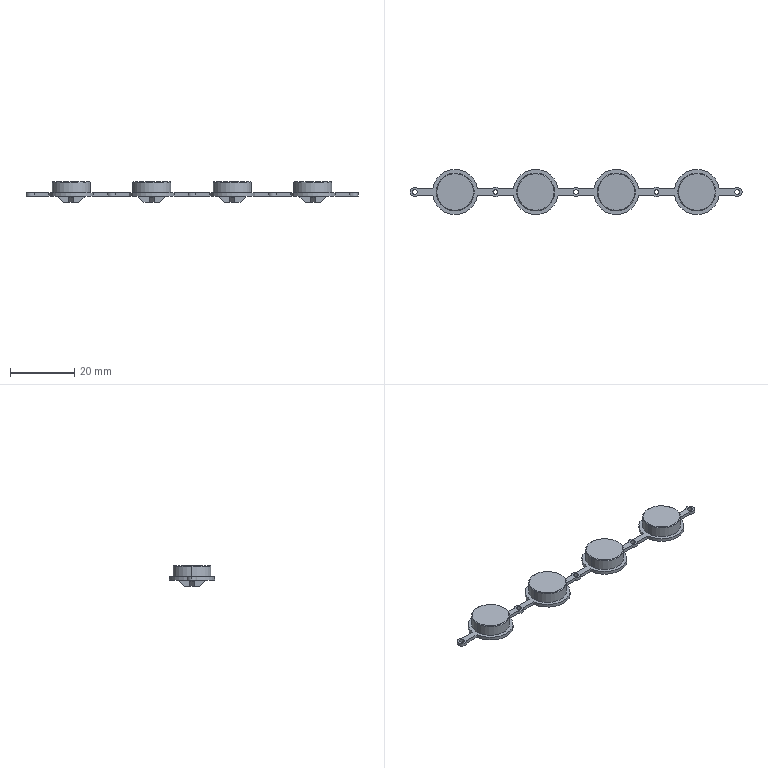Part | SolidWorks | features Chamfer 2, ICE 2, Extrusion 1 | 1 solid | 133 faces | box 103 x 14 x 6.5 mm | volume 2380 mm3 | plane 90 | cylinder 35 | cone 8 | commonest cylinder face diameters 1.5 x10 3 x9 11.8 x8 14 x8